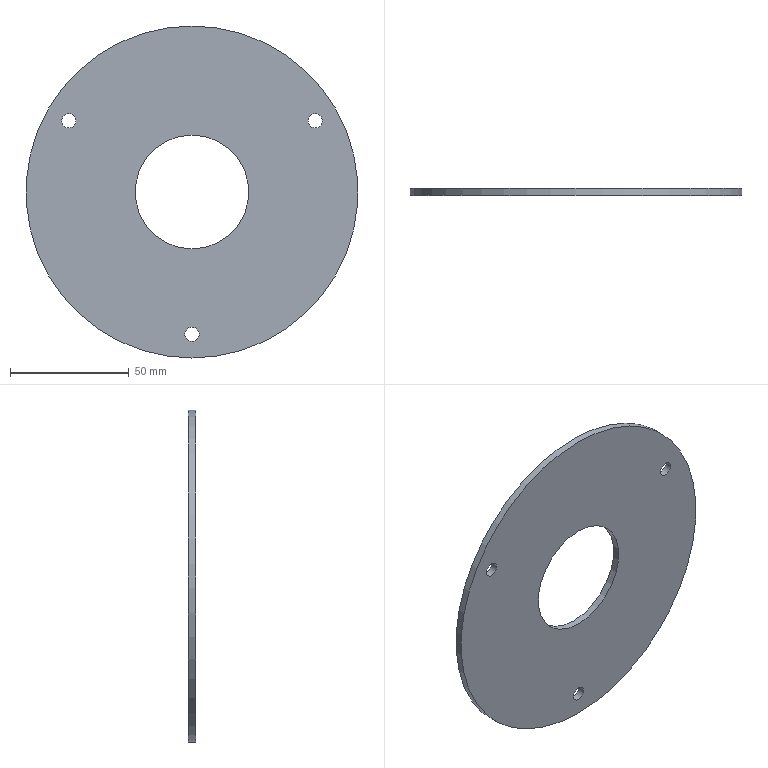Part | STEP file | JBJ-P-1018-02 | 1 solid | 7 faces | box 140 x 3 x 140 mm | volume 40498 mm3 | cylinder 5 | plane 2 | commonest cylinder face diameters 6 x3 48 x1 140 x1
STEP:
#1=CARTESIAN_POINT('',(51.962,3.,33.));
#2=VERTEX_POINT('',#1);
#3=CARTESIAN_POINT('',(51.962,3.,30.));
#4=DIRECTION('',(0.,1.,0.));
#5=DIRECTION('',(0.,0.,1.));
#6=AXIS2_PLACEMENT_3D('',#3,#4,#5);
#7=CIRCLE('',#6,3.);
#8=EDGE_CURVE('',#2,#2,#7,.T.);
#9=ORIENTED_EDGE('',*,*,#8,.F.);
#10=EDGE_LOOP('',(#9));
#11=FACE_BOUND('',#10,.T.);
#12=CARTESIAN_POINT('',(0.,3.,24.));
#13=VERTEX_POINT('',#12);
#14=CARTESIAN_POINT('',(0.,3.,0.));
#15=DIRECTION('',(0.,1.,0.));
#16=DIRECTION('',(0.,0.,1.));
#17=AXIS2_PLACEMENT_3D('',#14,#15,#16);
#18=CIRCLE('',#17,24.);
#19=EDGE_CURVE('',#13,#13,#18,.T.);
#20=ORIENTED_EDGE('',*,*,#19,.F.);
#21=EDGE_LOOP('',(#20));
#22=FACE_BOUND('',#21,.T.);
#23=CARTESIAN_POINT('',(0.,3.,70.));
#24=VERTEX_POINT('',#23);
#25=CARTESIAN_POINT('',(0.,3.,0.));
#26=DIRECTION('',(0.,1.,0.));
#27=DIRECTION('',(0.,0.,1.));
#28=AXIS2_PLACEMENT_3D('',#25,#26,#27);
#29=CIRCLE('',#28,70.);
#30=EDGE_CURVE('',#24,#24,#29,.T.);
#31=ORIENTED_EDGE('',*,*,#30,.T.);
#32=EDGE_LOOP('',(#31));
#33=FACE_OUTER_BOUND('',#32,.T.);
#34=CARTESIAN_POINT('',(0.,3.,-57.));
#35=VERTEX_POINT('',#34);
#36=CARTESIAN_POINT('',(0.,3.,-60.));
#37=DIRECTION('',(0.,1.,0.));
#38=DIRECTION('',(0.,0.,1.));
#39=AXIS2_PLACEMENT_3D('',#36,#37,#38);
#40=CIRCLE('',#39,3.);
#41=EDGE_CURVE('',#35,#35,#40,.T.);
#42=ORIENTED_EDGE('',*,*,#41,.F.);
#43=EDGE_LOOP('',(#42));
#44=FACE_BOUND('',#43,.T.);
#45=CARTESIAN_POINT('',(-51.962,3.,33.));
#46=VERTEX_POINT('',#45);
#47=CARTESIAN_POINT('',(-51.962,3.,30.));
#48=DIRECTION('',(0.,1.,0.));
#49=DIRECTION('',(0.,0.,1.));
#50=AXIS2_PLACEMENT_3D('',#47,#48,#49);
#51=CIRCLE('',#50,3.);
#52=EDGE_CURVE('',#46,#46,#51,.T.);
#53=ORIENTED_EDGE('',*,*,#52,.F.);
#54=EDGE_LOOP('',(#53));
#55=FACE_BOUND('',#54,.T.);
#56=CARTESIAN_POINT('',(0.,3.,0.));
#57=DIRECTION('',(0.,1.,0.));
#58=DIRECTION('',(0.,0.,1.));
#59=AXIS2_PLACEMENT_3D('',#56,#57,#58);
#60=PLANE('',#59);
#61=ADVANCED_FACE('',(#11,#22,#33,#44,#55),#60,.T.);
#62=CARTESIAN_POINT('',(0.,0.,70.));
#63=VERTEX_POINT('',#62);
#64=CARTESIAN_POINT('',(0.,0.,0.));
#65=DIRECTION('',(0.,1.,0.));
#66=DIRECTION('',(0.,0.,1.));
#67=AXIS2_PLACEMENT_3D('',#64,#65,#66);
#68=CIRCLE('',#67,70.);
#69=EDGE_CURVE('',#63,#63,#68,.T.);
#70=ORIENTED_EDGE('',*,*,#69,.F.);
#71=EDGE_LOOP('',(#70));
#72=FACE_OUTER_BOUND('',#71,.T.);
#73=CARTESIAN_POINT('',(0.,0.,24.));
#74=VERTEX_POINT('',#73);
#75=CARTESIAN_POINT('',(0.,0.,0.));
#76=DIRECTION('',(0.,1.,0.));
#77=DIRECTION('',(0.,0.,1.));
#78=AXIS2_PLACEMENT_3D('',#75,#76,#77);
#79=CIRCLE('',#78,24.);
#80=EDGE_CURVE('',#74,#74,#79,.T.);
#81=ORIENTED_EDGE('',*,*,#80,.T.);
#82=EDGE_LOOP('',(#81));
#83=FACE_BOUND('',#82,.T.);
#84=CARTESIAN_POINT('',(0.,0.,-57.));
#85=VERTEX_POINT('',#84);
#86=CARTESIAN_POINT('',(0.,0.,-60.));
#87=DIRECTION('',(0.,1.,0.));
#88=DIRECTION('',(0.,0.,1.));
#89=AXIS2_PLACEMENT_3D('',#86,#87,#88);
#90=CIRCLE('',#89,3.);
#91=EDGE_CURVE('',#85,#85,#90,.T.);
#92=ORIENTED_EDGE('',*,*,#91,.T.);
#93=EDGE_LOOP('',(#92));
#94=FACE_BOUND('',#93,.T.);
#95=CARTESIAN_POINT('',(51.962,0.,33.));
#96=VERTEX_POINT('',#95);
#97=CARTESIAN_POINT('',(51.962,0.,30.));
#98=DIRECTION('',(0.,1.,0.));
#99=DIRECTION('',(0.,0.,1.));
#100=AXIS2_PLACEMENT_3D('',#97,#98,#99);
#101=CIRCLE('',#100,3.);
#102=EDGE_CURVE('',#96,#96,#101,.T.);
#103=ORIENTED_EDGE('',*,*,#102,.T.);
#104=EDGE_LOOP('',(#103));
#105=FACE_BOUND('',#104,.T.);
#106=CARTESIAN_POINT('',(-51.962,0.,33.));
#107=VERTEX_POINT('',#106);
#108=CARTESIAN_POINT('',(-51.962,0.,30.));
#109=DIRECTION('',(0.,1.,0.));
#110=DIRECTION('',(0.,0.,1.));
#111=AXIS2_PLACEMENT_3D('',#108,#109,#110);
#112=CIRCLE('',#111,3.);
#113=EDGE_CURVE('',#107,#107,#112,.T.);
#114=ORIENTED_EDGE('',*,*,#113,.T.);
#115=EDGE_LOOP('',(#114));
#116=FACE_BOUND('',#115,.T.);
#117=CARTESIAN_POINT('',(0.,0.,0.));
#118=DIRECTION('',(0.,1.,0.));
#119=DIRECTION('',(0.,0.,1.));
#120=AXIS2_PLACEMENT_3D('',#117,#118,#119);
#121=PLANE('',#120);
#122=ADVANCED_FACE('',(#72,#83,#94,#105,#116),#121,.F.);
#123=ORIENTED_EDGE('',*,*,#30,.F.);
#124=EDGE_LOOP('',(#123));
#125=FACE_OUTER_BOUND('',#124,.T.);
#126=ORIENTED_EDGE('',*,*,#69,.T.);
#127=EDGE_LOOP('',(#126));
#128=FACE_OUTER_BOUND('',#127,.T.);
#129=CARTESIAN_POINT('',(0.,3.,0.));
#130=DIRECTION('',(0.,-1.,0.));
#131=DIRECTION('',(0.,0.,-1.));
#132=AXIS2_PLACEMENT_3D('',#129,#130,#131);
#133=CYLINDRICAL_SURFACE('',#132,70.);
#134=ADVANCED_FACE('',(#125,#128),#133,.T.);
#135=ORIENTED_EDGE('',*,*,#19,.T.);
#136=EDGE_LOOP('',(#135));
#137=FACE_OUTER_BOUND('',#136,.T.);
#138=ORIENTED_EDGE('',*,*,#80,.F.);
#139=EDGE_LOOP('',(#138));
#140=FACE_OUTER_BOUND('',#139,.T.);
#141=CARTESIAN_POINT('',(0.,3.,0.));
#142=DIRECTION('',(0.,-1.,0.));
#143=DIRECTION('',(0.,0.,-1.));
#144=AXIS2_PLACEMENT_3D('',#141,#142,#143);
#145=CYLINDRICAL_SURFACE('',#144,24.);
#146=ADVANCED_FACE('',(#137,#140),#145,.F.);
#147=ORIENTED_EDGE('',*,*,#41,.T.);
#148=EDGE_LOOP('',(#147));
#149=FACE_OUTER_BOUND('',#148,.T.);
#150=ORIENTED_EDGE('',*,*,#91,.F.);
#151=EDGE_LOOP('',(#150));
#152=FACE_OUTER_BOUND('',#151,.T.);
#153=CARTESIAN_POINT('',(0.,3.,-60.));
#154=DIRECTION('',(0.,-1.,0.));
#155=DIRECTION('',(0.,0.,-1.));
#156=AXIS2_PLACEMENT_3D('',#153,#154,#155);
#157=CYLINDRICAL_SURFACE('',#156,3.);
#158=ADVANCED_FACE('',(#149,#152),#157,.F.);
#159=ORIENTED_EDGE('',*,*,#8,.T.);
#160=EDGE_LOOP('',(#159));
#161=FACE_OUTER_BOUND('',#160,.T.);
#162=ORIENTED_EDGE('',*,*,#102,.F.);
#163=EDGE_LOOP('',(#162));
#164=FACE_OUTER_BOUND('',#163,.T.);
#165=CARTESIAN_POINT('',(51.962,3.,30.));
#166=DIRECTION('',(0.,-1.,0.));
#167=DIRECTION('',(0.,0.,-1.));
#168=AXIS2_PLACEMENT_3D('',#165,#166,#167);
#169=CYLINDRICAL_SURFACE('',#168,3.);
#170=ADVANCED_FACE('',(#161,#164),#169,.F.);
#171=ORIENTED_EDGE('',*,*,#52,.T.);
#172=EDGE_LOOP('',(#171));
#173=FACE_OUTER_BOUND('',#172,.T.);
#174=ORIENTED_EDGE('',*,*,#113,.F.);
#175=EDGE_LOOP('',(#174));
#176=FACE_OUTER_BOUND('',#175,.T.);
#177=CARTESIAN_POINT('',(-51.962,3.,30.));
#178=DIRECTION('',(0.,-1.,0.));
#179=DIRECTION('',(0.,0.,-1.));
#180=AXIS2_PLACEMENT_3D('',#177,#178,#179);
#181=CYLINDRICAL_SURFACE('',#180,3.);
#182=ADVANCED_FACE('',(#173,#176),#181,.F.);
#183=CLOSED_SHELL('',(#61,#122,#134,#146,#158,#170,#182));
#184=MANIFOLD_SOLID_BREP('',#183);
#185=CARTESIAN_POINT('',(0.,0.,0.));
#186=DIRECTION('',(0.,0.,1.));
#187=DIRECTION('',(1.,0.,0.));
#188=AXIS2_PLACEMENT_3D('',#185,#186,#187);
#189=(LENGTH_UNIT()NAMED_UNIT(*)SI_UNIT(.MILLI.,.METRE.));
#190=UNCERTAINTY_MEASURE_WITH_UNIT(LENGTH_MEASURE(0.00001),#189,'','');
#191=(NAMED_UNIT(*)PLANE_ANGLE_UNIT()SI_UNIT($,.RADIAN.));
#192=(NAMED_UNIT(*)SI_UNIT($,.STERADIAN.)SOLID_ANGLE_UNIT());
#193=(GEOMETRIC_REPRESENTATION_CONTEXT(3)GLOBAL_UNCERTAINTY_ASSIGNED_CONTEXT((#190))GLOBAL_UNIT_ASSIGNED_CONTEXT((#189,#191,#192))REPRESENTATION_CONTEXT('',''));
#194=ADVANCED_BREP_SHAPE_REPRESENTATION('',(#184,#188),#193);